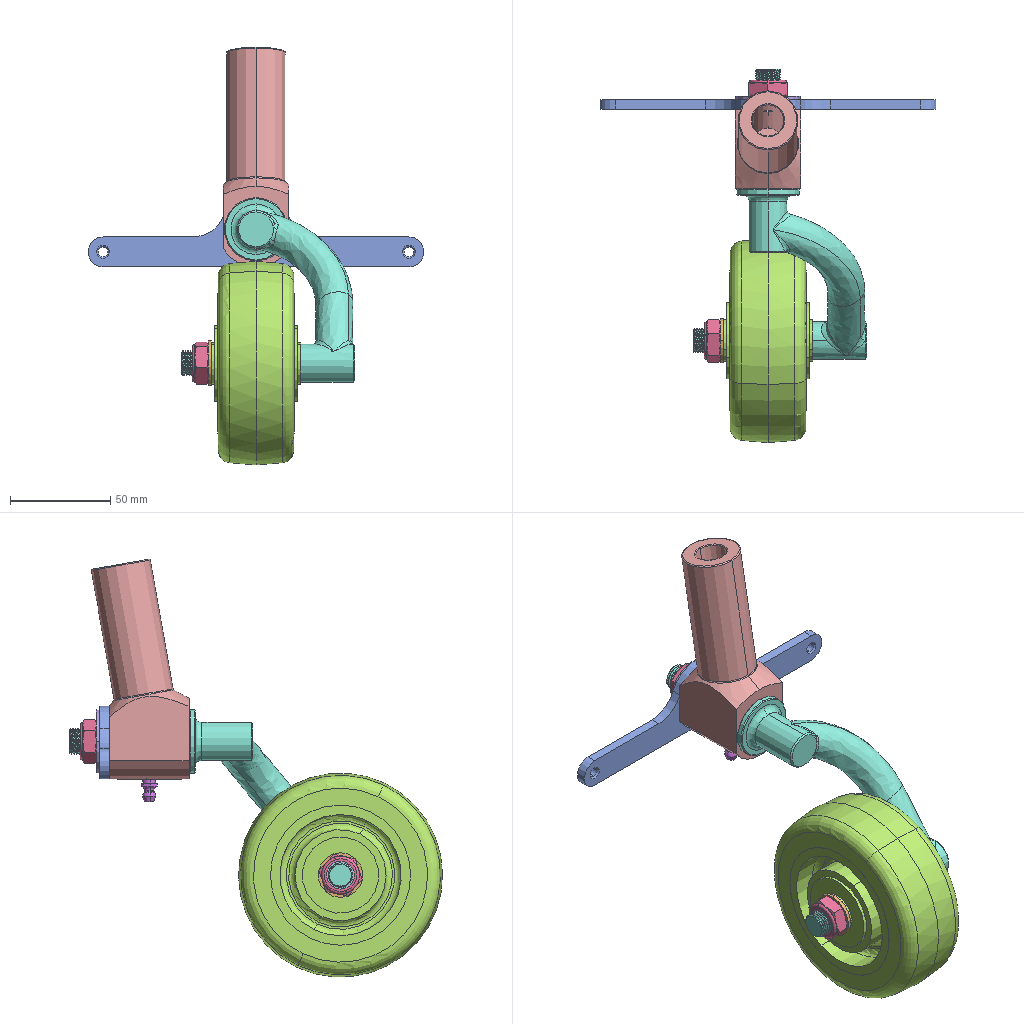Assembly | SolidWorks | 10 different items | 11 placed | box 167 x 186 x 208 mm
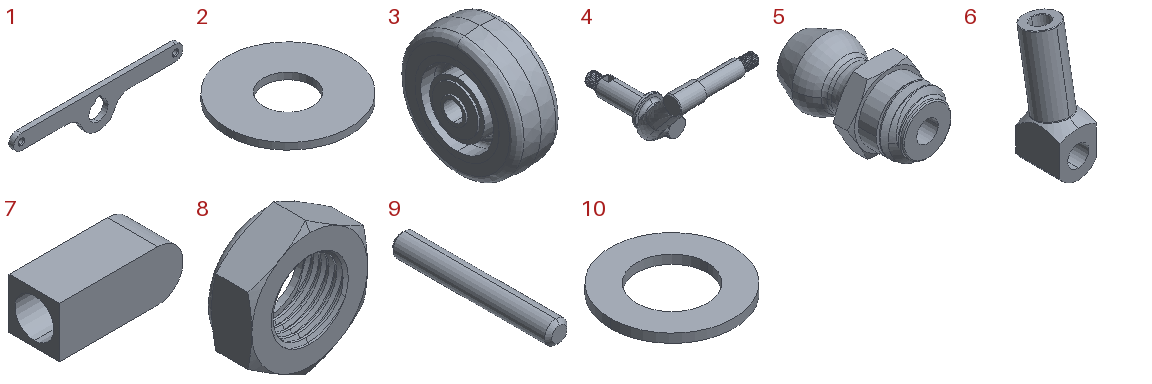Parts list (item | quantity | size | volume | features):
1 | x1 | 167.386 x 4.826 x 36.182 mm | 13483 mm3 | features Chamfer 1, Extrusion 1
2 | x1 | 32.004 x 32.004 x 1.753 mm | 1186 mm3 | features Extrusion 1
3 | x1 | 44.45 x 101.6 x 101.6 mm | 249789 mm3 | features Revolution 1
4 | x1 | 86.354 x 144.501 x 91.948 mm | 66693 mm3 | features ICE 7, Chamfer 5, Fillet 3, SweepThread 2, Extrusion 1, Revolution 1, Sweep 1
5 | x1 | 8.249 x 13.277 x 7.144 mm | 337.025 mm3 | features ICE 4, Revolution 3, Fillet 1, Helix 1, RevCut 1, Split 1, SweepCut 1
6 | x1 | 32.614 x 48.684 x 109.683 mm | 70811 mm3 | features ICE 6, Fillet 2, 3DProfileFeature 1, Extrusion 1, HoleWzd 1, RevCutThin 1
7 | x1 | 15.494 x 6.35 x 6.35 mm | 372.244 mm3 | features Extrusion 1, ICE 1, RevCut 1
8 | x2 | 19.05 x 7.938 x 21.997 mm | 1490 mm3 | features RevCut 4, Revolution 2, CombineBodies 1, Extrusion 1, LPattern 1
9 | x1 | 1.575 x 11.112 x 1.575 mm | 21.36 mm3 | features Chamfer 1, Extrusion 1
10 | x1 | 22.276 x 22.276 x 1.6 mm | 419.302 mm3 | features Extrusion 1
Mates (type | each side: item.copy, entity, surface, feature):
Coincident | assembly select_type:0 | assembly plane
PlanarAngleDim | assembly plane | assembly plane
Coincident | 6.1 face plane Boss-Extrude1 | 1.1 face plane Boss-Extrude1
Concentric | 6.1 face cylinder Cut-Extrude1 | 1.1 face cylinder Boss-Extrude1
Coincident | 3.1 plane | assembly plane
Concentric | 1.1 face cylinder Boss-Extrude1 | 7.1 face cylinder Boss-Extrude1
Concentric | 6.1 face cylinder Cut-Extrude1 | 4.1 face cylinder Boss-Extrude1
Coincident | 6.1 face plane Boss-Extrude1 | 4.1 face plane Revolve1
Concentric | 3.1 face cylinder Revolve1 | 4.1 face cylinder Boss-Extrude3
Coincident | 7.1 face plane Boss-Extrude1 | 4.1 face plane Cut-Extrude2
Width | 4.1 face plane Cut-Extrude2 | 4.1 face plane Cut-Extrude2 | 7.1 face plane Boss-Extrude1 | 7.1 face plane Boss-Extrude1
Coincident | 1.1 face plane Boss-Extrude1 | 2.1 face plane Boss-Extrude1
Concentric | 4.1 face cone Chamfer4 | 2.1 face cylinder Boss-Extrude1
Concentric | 3.1 face cylinder Revolve1 | 10.1 face cylinder Boss-Extrude1
Coincident | 3.1 face plane Revolve1 | 10.1 face plane Boss-Extrude1
Concentric | 4.1 face cylinder Cut-Extrude3 | 9.1 face cylinder Boss-Extrude1
Coincident | 4.1 face plane Boss-Extrude1 | 9.1 face plane Boss-Extrude1
Concentric | 2.1 face cylinder Boss-Extrude1 | 8.1 edge
Coincident | 2.1 face plane Boss-Extrude1 | 8.1 face plane Extrude1
Coincident | 10.1 face plane Boss-Extrude1 | 8.2 face plane Extrude1
Concentric | 10.1 face cylinder Boss-Extrude1 | 8.2 face cylinder Revolve2
Concentric | 6.1 face cylinder 1/4-28 Tapped Hole1 | 5.1 face cylinder Revolve1
Tangent | 6.1 face cylinder Cut-Extrude1 | 5.1 edge